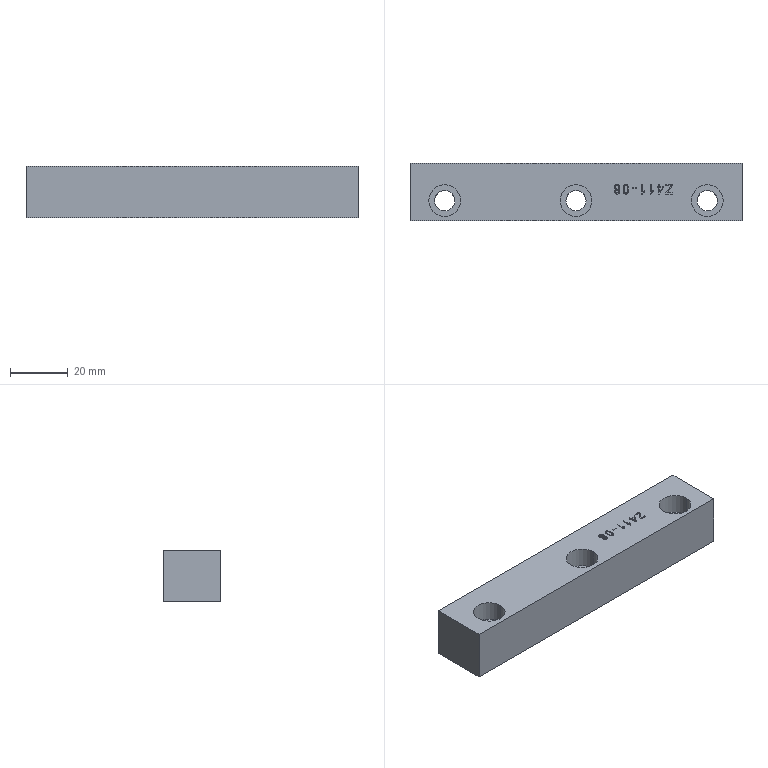Part | Creo | 1 solid | 133 faces | box 115 x 20 x 18 mm | volume 38131 mm3 | other 65 | plane 54 | cylinder 14 | commonest cylinder face diameters 7 x6 11 x6 1.666 x1 45.582 x1